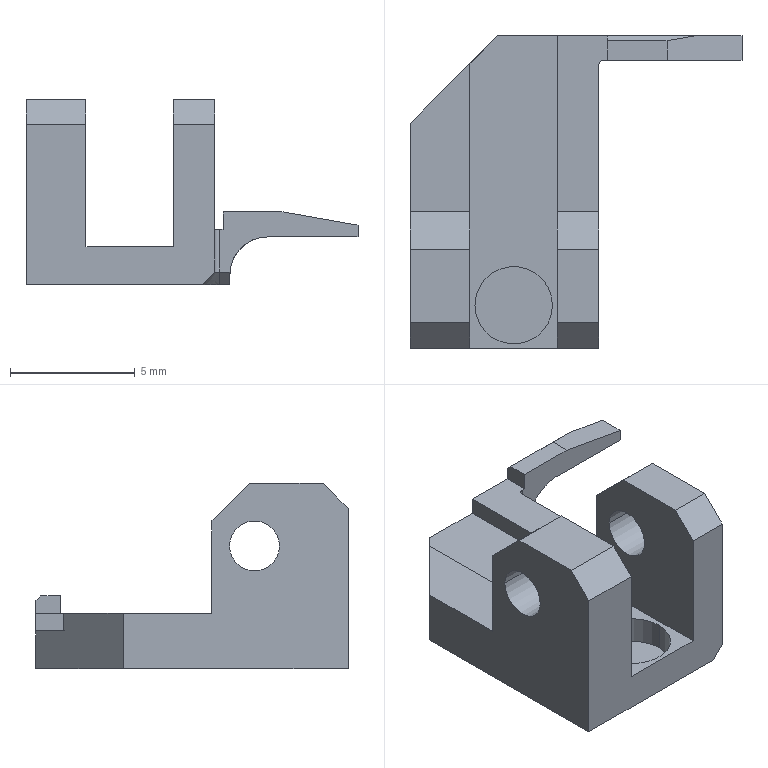Part | NX | 1 solid | 39 faces | box 13.281 x 12.5 x 7.405 mm | volume 256.212 mm3 | plane 30 | cylinder 8 | cone 1 | commonest cylinder face diameters 2 x4 3.1 x2 0.4 x1 3 x1
STEP:
#1=CARTESIAN_POINT('',(-42.479,-42.729,-0.8259));
#2=VERTEX_POINT('',#1);
#3=CARTESIAN_POINT('',(-42.479,-43.716,-0.8259));
#4=VERTEX_POINT('',#3);
#5=CARTESIAN_POINT('',(-42.479,-43.322,-0.8259));
#6=DIRECTION('',(0.,-1.,0.));
#7=VECTOR('',#6,1000.);
#8=LINE('',#5,#7);
#9=EDGE_CURVE('',#2,#4,#8,.T.);
#10=ORIENTED_EDGE('',*,*,#9,.T.);
#11=CARTESIAN_POINT('',(-42.479,-43.716,-1.297));
#12=VERTEX_POINT('',#11);
#13=CARTESIAN_POINT('',(-42.479,-43.716,-2.097));
#14=DIRECTION('',(0.,0.,1.));
#15=VECTOR('',#14,1000.);
#16=LINE('',#13,#15);
#17=EDGE_CURVE('',#12,#4,#16,.T.);
#18=ORIENTED_EDGE('',*,*,#17,.F.);
#19=CARTESIAN_POINT('',(-42.479,-42.729,-1.297));
#20=VERTEX_POINT('',#19);
#21=CARTESIAN_POINT('',(-42.479,-42.161,-1.297));
#22=DIRECTION('',(0.,1.,0.));
#23=VECTOR('',#22,1000.);
#24=LINE('',#21,#23);
#25=EDGE_CURVE('',#12,#20,#24,.T.);
#26=ORIENTED_EDGE('',*,*,#25,.T.);
#27=CARTESIAN_POINT('',(-42.479,-42.729,-2.097));
#28=DIRECTION('',(0.,0.,-1.));
#29=VECTOR('',#28,1000.);
#30=LINE('',#27,#29);
#31=EDGE_CURVE('',#2,#20,#30,.T.);
#32=ORIENTED_EDGE('',*,*,#31,.F.);
#33=EDGE_LOOP('',(#10,#18,#26,#32));
#34=FACE_BOUND('',#33,.T.);
#35=CARTESIAN_POINT('',(-42.479,-43.677,-2.097));
#36=DIRECTION('',(1.,0.,0.));
#37=DIRECTION('',(0.,0.,1.));
#38=AXIS2_PLACEMENT_3D('',#35,#36,#37);
#39=PLANE('',#38);
#40=ADVANCED_FACE('',(#34),#39,.T.);
#41=CARTESIAN_POINT('',(-47.879,-43.716,-0.9969));
#42=VERTEX_POINT('',#41);
#43=CARTESIAN_POINT('',(-47.879,-43.716,-0.2969));
#44=VERTEX_POINT('',#43);
#45=CARTESIAN_POINT('',(-47.879,-43.716,-2.097));
#46=DIRECTION('',(0.,0.,1.));
#47=VECTOR('',#46,1000.);
#48=LINE('',#45,#47);
#49=EDGE_CURVE('',#42,#44,#48,.T.);
#50=ORIENTED_EDGE('',*,*,#49,.T.);
#51=CARTESIAN_POINT('',(-47.879,-42.929,-0.2969));
#52=VERTEX_POINT('',#51);
#53=CARTESIAN_POINT('',(-47.879,-42.161,-0.2969));
#54=DIRECTION('',(0.,-1.,0.));
#55=VECTOR('',#54,1000.);
#56=LINE('',#53,#55);
#57=EDGE_CURVE('',#52,#44,#56,.T.);
#58=ORIENTED_EDGE('',*,*,#57,.F.);
#59=CARTESIAN_POINT('',(-47.879,-42.729,-0.4969));
#60=VERTEX_POINT('',#59);
#61=CARTESIAN_POINT('',(-47.879,-42.161,-1.065));
#62=DIRECTION('',(0.,0.7071,-0.7071));
#63=VECTOR('',#62,1000.);
#64=LINE('',#61,#63);
#65=EDGE_CURVE('',#52,#60,#64,.T.);
#66=ORIENTED_EDGE('',*,*,#65,.T.);
#67=CARTESIAN_POINT('',(-47.879,-42.729,-0.9969));
#68=VERTEX_POINT('',#67);
#69=CARTESIAN_POINT('',(-47.879,-42.729,-2.097));
#70=DIRECTION('',(0.,0.,-1.));
#71=VECTOR('',#70,1000.);
#72=LINE('',#69,#71);
#73=EDGE_CURVE('',#60,#68,#72,.T.);
#74=ORIENTED_EDGE('',*,*,#73,.T.);
#75=CARTESIAN_POINT('',(-47.879,-42.161,-0.9969));
#76=DIRECTION('',(0.,-1.,0.));
#77=VECTOR('',#76,1000.);
#78=LINE('',#75,#77);
#79=EDGE_CURVE('',#68,#42,#78,.T.);
#80=ORIENTED_EDGE('',*,*,#79,.T.);
#81=EDGE_LOOP('',(#50,#58,#66,#74,#80));
#82=FACE_BOUND('',#81,.T.);
#83=CARTESIAN_POINT('',(-47.879,-42.677,-2.097));
#84=DIRECTION('',(-1.,0.,0.));
#85=DIRECTION('',(0.,1.,0.));
#86=AXIS2_PLACEMENT_3D('',#83,#84,#85);
#87=PLANE('',#86);
#88=ADVANCED_FACE('',(#82),#87,.T.);
#89=CARTESIAN_POINT('',(-53.36,-43.829,-1.697));
#90=VERTEX_POINT('',#89);
#91=CARTESIAN_POINT('',(-53.36,-55.229,-1.697));
#92=VERTEX_POINT('',#91);
#93=CARTESIAN_POINT('',(-53.36,-42.161,-1.697));
#94=DIRECTION('',(0.,-1.,0.));
#95=VECTOR('',#94,1000.);
#96=LINE('',#93,#95);
#97=EDGE_CURVE('',#90,#92,#96,.T.);
#98=ORIENTED_EDGE('',*,*,#97,.F.);
#99=CARTESIAN_POINT('',(-53.36,-43.829,-0.9969));
#100=VERTEX_POINT('',#99);
#101=CARTESIAN_POINT('',(-53.36,-43.829,-2.097));
#102=DIRECTION('',(0.,0.,-1.));
#103=VECTOR('',#102,1000.);
#104=LINE('',#101,#103);
#105=EDGE_CURVE('',#100,#90,#104,.T.);
#106=ORIENTED_EDGE('',*,*,#105,.F.);
#107=CARTESIAN_POINT('',(-53.36,-49.779,-0.9969));
#108=VERTEX_POINT('',#107);
#109=CARTESIAN_POINT('',(-53.36,-42.161,-0.9969));
#110=DIRECTION('',(0.,-1.,0.));
#111=VECTOR('',#110,1000.);
#112=LINE('',#109,#111);
#113=EDGE_CURVE('',#100,#108,#112,.T.);
#114=ORIENTED_EDGE('',*,*,#113,.T.);
#115=CARTESIAN_POINT('',(-53.36,-49.779,2.703));
#116=VERTEX_POINT('',#115);
#117=CARTESIAN_POINT('',(-53.36,-49.779,-2.097));
#118=DIRECTION('',(0.,0.,-1.));
#119=VECTOR('',#118,1000.);
#120=LINE('',#117,#119);
#121=EDGE_CURVE('',#116,#108,#120,.T.);
#122=ORIENTED_EDGE('',*,*,#121,.F.);
#123=CARTESIAN_POINT('',(-53.36,-51.279,4.203));
#124=VERTEX_POINT('',#123);
#125=CARTESIAN_POINT('',(-53.36,-44.979,-2.097));
#126=DIRECTION('',(0.,-0.7071,0.7071));
#127=VECTOR('',#126,1000.);
#128=LINE('',#125,#127);
#129=EDGE_CURVE('',#116,#124,#128,.T.);
#130=ORIENTED_EDGE('',*,*,#129,.T.);
#131=CARTESIAN_POINT('',(-53.36,-54.229,4.203));
#132=VERTEX_POINT('',#131);
#133=CARTESIAN_POINT('',(-53.36,-42.161,4.203));
#134=DIRECTION('',(0.,1.,0.));
#135=VECTOR('',#134,1000.);
#136=LINE('',#133,#135);
#137=EDGE_CURVE('',#132,#124,#136,.T.);
#138=ORIENTED_EDGE('',*,*,#137,.F.);
#139=CARTESIAN_POINT('',(-53.36,-55.229,3.203));
#140=VERTEX_POINT('',#139);
#141=CARTESIAN_POINT('',(-53.36,-60.529,-2.097));
#142=DIRECTION('',(0.,-0.7071,-0.7071));
#143=VECTOR('',#142,1000.);
#144=LINE('',#141,#143);
#145=EDGE_CURVE('',#132,#140,#144,.T.);
#146=ORIENTED_EDGE('',*,*,#145,.T.);
#147=CARTESIAN_POINT('',(-53.36,-55.229,-2.097));
#148=DIRECTION('',(0.,0.,1.));
#149=VECTOR('',#148,1000.);
#150=LINE('',#147,#149);
#151=EDGE_CURVE('',#92,#140,#150,.T.);
#152=ORIENTED_EDGE('',*,*,#151,.F.);
#153=EDGE_LOOP('',(#98,#106,#114,#122,#130,#138,#146,#152));
#154=FACE_BOUND('',#153,.T.);
#155=CARTESIAN_POINT('',(-53.36,-50.479,1.703));
#156=VERTEX_POINT('',#155);
#157=CARTESIAN_POINT('',(-53.36,-52.479,1.703));
#158=VERTEX_POINT('',#157);
#159=CARTESIAN_POINT('',(-53.36,-51.479,1.703));
#160=DIRECTION('',(-1.,0.,0.));
#161=DIRECTION('',(0.,-1.,0.));
#162=AXIS2_PLACEMENT_3D('',#159,#160,#161);
#163=CIRCLE('',#162,1.);
#164=EDGE_CURVE('',#156,#158,#163,.T.);
#165=ORIENTED_EDGE('',*,*,#164,.T.);
#166=CARTESIAN_POINT('',(-53.36,-51.479,1.703));
#167=DIRECTION('',(-1.,0.,0.));
#168=DIRECTION('',(0.,-1.,0.));
#169=AXIS2_PLACEMENT_3D('',#166,#167,#168);
#170=CIRCLE('',#169,1.);
#171=EDGE_CURVE('',#158,#156,#170,.T.);
#172=ORIENTED_EDGE('',*,*,#171,.T.);
#173=EDGE_LOOP('',(#165,#172));
#174=FACE_BOUND('',#173,.T.);
#175=CARTESIAN_POINT('',(-53.36,-41.455,-0.9969));
#176=DIRECTION('',(-1.,0.,0.));
#177=DIRECTION('',(0.,0.,1.));
#178=AXIS2_PLACEMENT_3D('',#175,#176,#177);
#179=PLANE('',#178);
#180=ADVANCED_FACE('',(#154,#174),#179,.F.);
#181=CARTESIAN_POINT('',(-49.86,-42.729,-1.697));
#182=VERTEX_POINT('',#181);
#183=CARTESIAN_POINT('',(-52.26,-42.729,-1.697));
#184=VERTEX_POINT('',#183);
#185=CARTESIAN_POINT('',(-49.458,-42.729,-1.697));
#186=DIRECTION('',(-1.,0.,0.));
#187=VECTOR('',#186,1000.);
#188=LINE('',#185,#187);
#189=EDGE_CURVE('',#182,#184,#188,.T.);
#190=ORIENTED_EDGE('',*,*,#189,.F.);
#191=CARTESIAN_POINT('',(-49.86,-42.729,-0.9969));
#192=VERTEX_POINT('',#191);
#193=CARTESIAN_POINT('',(-49.86,-42.729,-2.097));
#194=DIRECTION('',(0.,0.,-1.));
#195=VECTOR('',#194,1000.);
#196=LINE('',#193,#195);
#197=EDGE_CURVE('',#192,#182,#196,.T.);
#198=ORIENTED_EDGE('',*,*,#197,.F.);
#199=CARTESIAN_POINT('',(-49.458,-42.729,-0.9969));
#200=DIRECTION('',(-1.,0.,0.));
#201=VECTOR('',#200,1000.);
#202=LINE('',#199,#201);
#203=EDGE_CURVE('',#68,#192,#202,.T.);
#204=ORIENTED_EDGE('',*,*,#203,.F.);
#205=ORIENTED_EDGE('',*,*,#73,.F.);
#206=CARTESIAN_POINT('',(-44.345,-42.729,-0.4969));
#207=VERTEX_POINT('',#206);
#208=CARTESIAN_POINT('',(-49.458,-42.729,-0.4969));
#209=DIRECTION('',(1.,0.,0.));
#210=VECTOR('',#209,1000.);
#211=LINE('',#208,#210);
#212=EDGE_CURVE('',#60,#207,#211,.T.);
#213=ORIENTED_EDGE('',*,*,#212,.T.);
#214=CARTESIAN_POINT('',(-49.458,-42.729,0.4047));
#215=DIRECTION('',(0.9848,0.,-0.1736));
#216=VECTOR('',#215,1000.);
#217=LINE('',#214,#216);
#218=EDGE_CURVE('',#207,#2,#217,.T.);
#219=ORIENTED_EDGE('',*,*,#218,.T.);
#220=ORIENTED_EDGE('',*,*,#31,.T.);
#221=CARTESIAN_POINT('',(-46.102,-42.729,-1.297));
#222=VERTEX_POINT('',#221);
#223=CARTESIAN_POINT('',(-49.458,-42.729,-1.297));
#224=DIRECTION('',(-1.,0.,0.));
#225=VECTOR('',#224,1000.);
#226=LINE('',#223,#225);
#227=EDGE_CURVE('',#20,#222,#226,.T.);
#228=ORIENTED_EDGE('',*,*,#227,.T.);
#229=CARTESIAN_POINT('',(-47.602,-42.729,-2.797));
#230=VERTEX_POINT('',#229);
#231=CARTESIAN_POINT('',(-46.102,-42.729,-2.797));
#232=DIRECTION('',(0.,1.,0.));
#233=DIRECTION('',(-1.,0.,0.));
#234=AXIS2_PLACEMENT_3D('',#231,#232,#233);
#235=CIRCLE('',#234,1.5);
#236=EDGE_CURVE('',#230,#222,#235,.T.);
#237=ORIENTED_EDGE('',*,*,#236,.F.);
#238=CARTESIAN_POINT('',(-47.602,-42.729,-3.201));
#239=VERTEX_POINT('',#238);
#240=CARTESIAN_POINT('',(-47.602,-42.729,-2.097));
#241=DIRECTION('',(0.,0.,1.));
#242=VECTOR('',#241,1000.);
#243=LINE('',#240,#242);
#244=EDGE_CURVE('',#239,#230,#243,.T.);
#245=ORIENTED_EDGE('',*,*,#244,.F.);
#246=CARTESIAN_POINT('',(-52.26,-42.729,-3.201));
#247=VERTEX_POINT('',#246);
#248=CARTESIAN_POINT('',(-49.458,-42.729,-3.201));
#249=DIRECTION('',(-1.,0.,0.));
#250=VECTOR('',#249,1000.);
#251=LINE('',#248,#250);
#252=EDGE_CURVE('',#239,#247,#251,.T.);
#253=ORIENTED_EDGE('',*,*,#252,.T.);
#254=CARTESIAN_POINT('',(-52.26,-42.729,-2.097));
#255=DIRECTION('',(0.,0.,1.));
#256=VECTOR('',#255,1000.);
#257=LINE('',#254,#256);
#258=EDGE_CURVE('',#247,#184,#257,.T.);
#259=ORIENTED_EDGE('',*,*,#258,.T.);
#260=EDGE_LOOP('',(#190,#198,#204,#205,#213,#219,#220,#228,#237,#245,#253,#259));
#261=FACE_BOUND('',#260,.T.);
#262=CARTESIAN_POINT('',(-40.479,-42.729,-2.097));
#263=DIRECTION('',(0.,1.,0.));
#264=DIRECTION('',(0.,0.,-1.));
#265=AXIS2_PLACEMENT_3D('',#262,#263,#264);
#266=PLANE('',#265);
#267=ADVANCED_FACE('',(#261),#266,.T.);
#268=CARTESIAN_POINT('',(-48.01,-43.716,-2.701));
#269=VERTEX_POINT('',#268);
#270=CARTESIAN_POINT('',(-47.599,-43.716,-2.701));
#271=VERTEX_POINT('',#270);
#272=CARTESIAN_POINT('',(-47.806,-43.716,-2.701));
#273=DIRECTION('',(1.,0.,0.));
#274=VECTOR('',#273,1000.);
#275=LINE('',#272,#274);
#276=EDGE_CURVE('',#269,#271,#275,.T.);
#277=ORIENTED_EDGE('',*,*,#276,.T.);
#278=CARTESIAN_POINT('',(-46.102,-43.716,-1.297));
#279=VERTEX_POINT('',#278);
#280=CARTESIAN_POINT('',(-46.102,-43.716,-2.797));
#281=DIRECTION('',(0.,1.,0.));
#282=DIRECTION('',(-1.,0.,0.));
#283=AXIS2_PLACEMENT_3D('',#280,#281,#282);
#284=CIRCLE('',#283,1.5);
#285=EDGE_CURVE('',#271,#279,#284,.T.);
#286=ORIENTED_EDGE('',*,*,#285,.T.);
#287=CARTESIAN_POINT('',(-49.458,-43.716,-1.297));
#288=DIRECTION('',(1.,0.,0.));
#289=VECTOR('',#288,1000.);
#290=LINE('',#287,#289);
#291=EDGE_CURVE('',#279,#12,#290,.T.);
#292=ORIENTED_EDGE('',*,*,#291,.T.);
#293=ORIENTED_EDGE('',*,*,#17,.T.);
#294=CARTESIAN_POINT('',(-45.479,-43.716,-0.2969));
#295=VERTEX_POINT('',#294);
#296=CARTESIAN_POINT('',(-49.458,-43.716,0.4047));
#297=DIRECTION('',(-0.9848,0.,0.1736));
#298=VECTOR('',#297,1000.);
#299=LINE('',#296,#298);
#300=EDGE_CURVE('',#4,#295,#299,.T.);
#301=ORIENTED_EDGE('',*,*,#300,.T.);
#302=CARTESIAN_POINT('',(-49.458,-43.716,-0.2969));
#303=DIRECTION('',(-1.,0.,0.));
#304=VECTOR('',#303,1000.);
#305=LINE('',#302,#304);
#306=EDGE_CURVE('',#295,#44,#305,.T.);
#307=ORIENTED_EDGE('',*,*,#306,.T.);
#308=ORIENTED_EDGE('',*,*,#49,.F.);
#309=CARTESIAN_POINT('',(-48.01,-43.716,-0.9969));
#310=VERTEX_POINT('',#309);
#311=CARTESIAN_POINT('',(-49.458,-43.716,-0.9969));
#312=DIRECTION('',(1.,0.,0.));
#313=VECTOR('',#312,1000.);
#314=LINE('',#311,#313);
#315=EDGE_CURVE('',#310,#42,#314,.T.);
#316=ORIENTED_EDGE('',*,*,#315,.F.);
#317=CARTESIAN_POINT('',(-48.01,-43.716,-2.097));
#318=DIRECTION('',(0.,0.,-1.));
#319=VECTOR('',#318,1000.);
#320=LINE('',#317,#319);
#321=EDGE_CURVE('',#310,#269,#320,.T.);
#322=ORIENTED_EDGE('',*,*,#321,.T.);
#323=EDGE_LOOP('',(#277,#286,#292,#293,#301,#307,#308,#316,#322));
#324=FACE_BOUND('',#323,.T.);
#325=CARTESIAN_POINT('',(-49.857,-43.716,-2.975));
#326=DIRECTION('',(0.,-1.,0.));
#327=DIRECTION('',(-1.,0.,0.));
#328=AXIS2_PLACEMENT_3D('',#325,#326,#327);
#329=PLANE('',#328);
#330=ADVANCED_FACE('',(#324),#329,.T.);
#331=CARTESIAN_POINT('',(-48.21,-55.229,-2.701));
#332=VERTEX_POINT('',#331);
#333=CARTESIAN_POINT('',(-48.21,-55.229,3.203));
#334=VERTEX_POINT('',#333);
#335=CARTESIAN_POINT('',(-48.21,-55.229,-2.097));
#336=DIRECTION('',(0.,0.,1.));
#337=VECTOR('',#336,1000.);
#338=LINE('',#335,#337);
#339=EDGE_CURVE('',#332,#334,#338,.T.);
#340=ORIENTED_EDGE('',*,*,#339,.T.);
#341=CARTESIAN_POINT('',(-49.86,-55.229,3.203));
#342=VERTEX_POINT('',#341);
#343=CARTESIAN_POINT('',(-49.035,-55.229,3.203));
#344=DIRECTION('',(1.,0.,0.));
#345=VECTOR('',#344,1000.);
#346=LINE('',#343,#345);
#347=EDGE_CURVE('',#342,#334,#346,.T.);
#348=ORIENTED_EDGE('',*,*,#347,.F.);
#349=CARTESIAN_POINT('',(-49.86,-55.229,-1.697));
#350=VERTEX_POINT('',#349);
#351=CARTESIAN_POINT('',(-49.86,-55.229,-2.097));
#352=DIRECTION('',(0.,0.,-1.));
#353=VECTOR('',#352,1000.);
#354=LINE('',#351,#353);
#355=EDGE_CURVE('',#342,#350,#354,.T.);
#356=ORIENTED_EDGE('',*,*,#355,.T.);
#357=CARTESIAN_POINT('',(-49.458,-55.229,-1.697));
#358=DIRECTION('',(-1.,0.,0.));
#359=VECTOR('',#358,1000.);
#360=LINE('',#357,#359);
#361=EDGE_CURVE('',#350,#92,#360,.T.);
#362=ORIENTED_EDGE('',*,*,#361,.T.);
#363=ORIENTED_EDGE('',*,*,#151,.T.);
#364=CARTESIAN_POINT('',(-55.76,-55.229,3.203));
#365=VERTEX_POINT('',#364);
#366=CARTESIAN_POINT('',(-49.458,-55.229,3.203));
#367=DIRECTION('',(1.,0.,0.));
#368=VECTOR('',#367,1000.);
#369=LINE('',#366,#368);
#370=EDGE_CURVE('',#365,#140,#369,.T.);
#371=ORIENTED_EDGE('',*,*,#370,.F.);
#372=CARTESIAN_POINT('',(-55.76,-55.229,-3.201));
#373=VERTEX_POINT('',#372);
#374=CARTESIAN_POINT('',(-55.76,-55.229,-2.097));
#375=DIRECTION('',(0.,0.,-1.));
#376=VECTOR('',#375,1000.);
#377=LINE('',#374,#376);
#378=EDGE_CURVE('',#365,#373,#377,.T.);
#379=ORIENTED_EDGE('',*,*,#378,.T.);
#380=CARTESIAN_POINT('',(-48.71,-55.229,-3.201));
#381=VERTEX_POINT('',#380);
#382=CARTESIAN_POINT('',(-49.458,-55.229,-3.201));
#383=DIRECTION('',(1.,0.,0.));
#384=VECTOR('',#383,1000.);
#385=LINE('',#382,#384);
#386=EDGE_CURVE('',#373,#381,#385,.T.);
#387=ORIENTED_EDGE('',*,*,#386,.T.);
#388=CARTESIAN_POINT('',(-49.458,-55.229,-3.949));
#389=DIRECTION('',(0.7071,0.,0.7071));
#390=VECTOR('',#389,1000.);
#391=LINE('',#388,#390);
#392=EDGE_CURVE('',#381,#332,#391,.T.);
#393=ORIENTED_EDGE('',*,*,#392,.T.);
#394=EDGE_LOOP('',(#340,#348,#356,#362,#363,#371,#379,#387,#393));
#395=FACE_BOUND('',#394,.T.);
#396=CARTESIAN_POINT('',(-46.479,-55.229,-2.097));
#397=DIRECTION('',(0.,-1.,0.));
#398=DIRECTION('',(-1.,0.,0.));
#399=AXIS2_PLACEMENT_3D('',#396,#397,#398);
#400=PLANE('',#399);
#401=ADVANCED_FACE('',(#395),#400,.T.);
#402=CARTESIAN_POINT('',(-47.602,-43.62,-2.797));
#403=VERTEX_POINT('',#402);
#404=CARTESIAN_POINT('',(-47.602,-42.161,-2.797));
#405=DIRECTION('',(0.,1.,0.));
#406=VECTOR('',#405,1000.);
#407=LINE('',#404,#406);
#408=EDGE_CURVE('',#403,#230,#407,.T.);
#409=ORIENTED_EDGE('',*,*,#408,.F.);
#410=CARTESIAN_POINT('',(-47.602,-43.216,-3.201));
#411=VERTEX_POINT('',#410);
#412=CARTESIAN_POINT('',(-47.602,-44.32,-2.097));
#413=DIRECTION('',(0.,0.7071,-0.7071));
#414=VECTOR('',#413,1000.);
#415=LINE('',#412,#414);
#416=EDGE_CURVE('',#403,#411,#415,.T.);
#417=ORIENTED_EDGE('',*,*,#416,.T.);
#418=CARTESIAN_POINT('',(-47.602,-42.161,-3.201));
#419=DIRECTION('',(0.,-1.,0.));
#420=VECTOR('',#419,1000.);
#421=LINE('',#418,#420);
#422=EDGE_CURVE('',#239,#411,#421,.T.);
#423=ORIENTED_EDGE('',*,*,#422,.F.);
#424=ORIENTED_EDGE('',*,*,#244,.T.);
#425=EDGE_LOOP('',(#409,#417,#423,#424));
#426=FACE_BOUND('',#425,.T.);
#427=CARTESIAN_POINT('',(-47.602,-42.161,-2.747));
#428=DIRECTION('',(-1.,0.,0.));
#429=DIRECTION('',(0.,0.,1.));
#430=AXIS2_PLACEMENT_3D('',#427,#428,#429);
#431=PLANE('',#430);
#432=ADVANCED_FACE('',(#426),#431,.F.);
#433=ORIENTED_EDGE('',*,*,#164,.F.);
#434=CARTESIAN_POINT('',(-55.76,-50.479,1.703));
#435=VERTEX_POINT('',#434);
#436=CARTESIAN_POINT('',(-40.131,-50.479,1.703));
#437=DIRECTION('',(-1.,0.,0.));
#438=VECTOR('',#437,1000.);
#439=LINE('',#436,#438);
#440=EDGE_CURVE('',#435,#156,#439,.F.);
#441=ORIENTED_EDGE('',*,*,#440,.F.);
#442=CARTESIAN_POINT('',(-55.76,-52.479,1.703));
#443=VERTEX_POINT('',#442);
#444=CARTESIAN_POINT('',(-55.76,-51.479,1.703));
#445=DIRECTION('',(-1.,0.,0.));
#446=DIRECTION('',(0.,-1.,0.));
#447=AXIS2_PLACEMENT_3D('',#444,#445,#446);
#448=CIRCLE('',#447,1.);
#449=EDGE_CURVE('',#435,#443,#448,.T.);
#450=ORIENTED_EDGE('',*,*,#449,.T.);
#451=CARTESIAN_POINT('',(-40.131,-52.479,1.703));
#452=DIRECTION('',(-1.,0.,0.));
#453=VECTOR('',#452,1000.);
#454=LINE('',#451,#453);
#455=EDGE_CURVE('',#443,#158,#454,.F.);
#456=ORIENTED_EDGE('',*,*,#455,.T.);
#457=EDGE_LOOP('',(#433,#441,#450,#456));
#458=FACE_BOUND('',#457,.T.);
#459=CARTESIAN_POINT('',(-40.131,-51.479,1.703));
#460=DIRECTION('',(-1.,0.,0.));
#461=DIRECTION('',(0.,-1.,0.));
#462=AXIS2_PLACEMENT_3D('',#459,#460,#461);
#463=CYLINDRICAL_SURFACE('',#462,1.);
#464=ADVANCED_FACE('',(#458),#463,.F.);
#465=CARTESIAN_POINT('',(-48.21,-43.916,-2.701));
#466=VERTEX_POINT('',#465);
#467=CARTESIAN_POINT('',(-48.01,-43.916,-2.701));
#468=DIRECTION('',(0.,0.,-1.));
#469=DIRECTION('',(-1.,0.,0.));
#470=AXIS2_PLACEMENT_3D('',#467,#468,#469);
#471=CIRCLE('',#470,0.2);
#472=EDGE_CURVE('',#466,#269,#471,.T.);
#473=ORIENTED_EDGE('',*,*,#472,.T.);
#474=ORIENTED_EDGE('',*,*,#321,.F.);
#475=CARTESIAN_POINT('',(-48.21,-43.916,-0.9969));
#476=VERTEX_POINT('',#475);
#477=CARTESIAN_POINT('',(-48.01,-43.916,-0.9969));
#478=DIRECTION('',(0.,0.,-1.));
#479=DIRECTION('',(-1.,0.,0.));
#480=AXIS2_PLACEMENT_3D('',#477,#478,#479);
#481=CIRCLE('',#480,0.2);
#482=EDGE_CURVE('',#476,#310,#481,.T.);
#483=ORIENTED_EDGE('',*,*,#482,.F.);
#484=CARTESIAN_POINT('',(-48.21,-43.916,-2.097));
#485=DIRECTION('',(0.,0.,-1.));
#486=VECTOR('',#485,1000.);
#487=LINE('',#484,#486);
#488=EDGE_CURVE('',#476,#466,#487,.T.);
#489=ORIENTED_EDGE('',*,*,#488,.T.);
#490=EDGE_LOOP('',(#473,#474,#483,#489));
#491=FACE_BOUND('',#490,.T.);
#492=CARTESIAN_POINT('',(-48.01,-43.916,-2.097));
#493=DIRECTION('',(0.,0.,-1.));
#494=DIRECTION('',(-1.,0.,0.));
#495=AXIS2_PLACEMENT_3D('',#492,#493,#494);
#496=CYLINDRICAL_SURFACE('',#495,0.2);
#497=ADVANCED_FACE('',(#491),#496,.F.);
#498=ORIENTED_EDGE('',*,*,#276,.F.);
#499=CARTESIAN_POINT('',(-48.01,-43.216,-3.201));
#500=VERTEX_POINT('',#499);
#501=CARTESIAN_POINT('',(-48.01,-43.716,-2.701));
#502=DIRECTION('',(0.,0.7071,-0.7071));
#503=VECTOR('',#502,1000.);
#504=LINE('',#501,#503);
#505=EDGE_CURVE('',#269,#500,#504,.T.);
#506=ORIENTED_EDGE('',*,*,#505,.T.);
#507=CARTESIAN_POINT('',(-47.806,-43.216,-3.201));
#508=DIRECTION('',(1.,0.,0.));
#509=VECTOR('',#508,1000.);
#510=LINE('',#507,#509);
#511=EDGE_CURVE('',#500,#411,#510,.T.);
#512=ORIENTED_EDGE('',*,*,#511,.T.);
#513=ORIENTED_EDGE('',*,*,#416,.F.);
#514=CARTESIAN_POINT('',(-47.599,-43.716,-2.701));
#515=CARTESIAN_POINT('',(-47.601,-43.684,-2.733));
#516=CARTESIAN_POINT('',(-47.602,-43.652,-2.765));
#517=CARTESIAN_POINT('',(-47.602,-43.62,-2.797));
#518=(BOUNDED_CURVE()B_SPLINE_CURVE(3,(#514,#515,#516,#517),.UNSPECIFIED.,.F.,.F.)B_SPLINE_CURVE_WITH_KNOTS((4,4),(4.649,4.712),.UNSPECIFIED.)CURVE()GEOMETRIC_REPRESENTATION_ITEM()RATIONAL_B_SPLINE_CURVE((1.,0.9997,0.9997,1.))REPRESENTATION_ITEM(''));
#519=EDGE_CURVE('',#271,#403,#518,.T.);
#520=ORIENTED_EDGE('',*,*,#519,.F.);
#521=EDGE_LOOP('',(#498,#506,#512,#513,#520));
#522=FACE_BOUND('',#521,.T.);
#523=CARTESIAN_POINT('',(-47.806,-43.466,-2.951));
#524=DIRECTION('',(0.,-0.7071,-0.7071));
#525=DIRECTION('',(0.,-0.7071,0.7071));
#526=AXIS2_PLACEMENT_3D('',#523,#524,#525);
#527=PLANE('',#526);
#528=ADVANCED_FACE('',(#522),#527,.T.);
#529=ORIENTED_EDGE('',*,*,#472,.F.);
#530=CARTESIAN_POINT('',(-48.71,-43.916,-3.201));
#531=VERTEX_POINT('',#530);
#532=CARTESIAN_POINT('',(-48.21,-43.916,-2.701));
#533=DIRECTION('',(-0.7071,0.,-0.7071));
#534=VECTOR('',#533,1000.);
#535=LINE('',#532,#534);
#536=EDGE_CURVE('',#466,#531,#535,.T.);
#537=ORIENTED_EDGE('',*,*,#536,.T.);
#538=CARTESIAN_POINT('',(-48.01,-43.916,-3.201));
#539=DIRECTION('',(0.,0.,-1.));
#540=DIRECTION('',(-1.,0.,0.));
#541=AXIS2_PLACEMENT_3D('',#538,#539,#540);
#542=CIRCLE('',#541,0.7);
#543=EDGE_CURVE('',#531,#500,#542,.T.);
#544=ORIENTED_EDGE('',*,*,#543,.T.);
#545=ORIENTED_EDGE('',*,*,#505,.F.);
#546=EDGE_LOOP('',(#529,#537,#544,#545));
#547=FACE_BOUND('',#546,.T.);
#548=CARTESIAN_POINT('',(-48.01,-43.916,-2.701));
#549=DIRECTION('',(0.,0.,-1.));
#550=DIRECTION('',(-1.,0.,0.));
#551=AXIS2_PLACEMENT_3D('',#548,#549,#550);
#552=CONICAL_SURFACE('',#551,0.2,0.7854);
#553=ADVANCED_FACE('',(#547),#552,.F.);
#554=ORIENTED_EDGE('',*,*,#408,.T.);
#555=ORIENTED_EDGE('',*,*,#236,.T.);
#556=CARTESIAN_POINT('',(-46.102,-42.161,-1.297));
#557=DIRECTION('',(0.,1.,0.));
#558=VECTOR('',#557,1000.);
#559=LINE('',#556,#558);
#560=EDGE_CURVE('',#279,#222,#559,.T.);
#561=ORIENTED_EDGE('',*,*,#560,.F.);
#562=ORIENTED_EDGE('',*,*,#285,.F.);
#563=ORIENTED_EDGE('',*,*,#519,.T.);
#564=EDGE_LOOP('',(#554,#555,#561,#562,#563));
#565=FACE_BOUND('',#564,.T.);
#566=CARTESIAN_POINT('',(-46.102,-42.161,-2.797));
#567=DIRECTION('',(0.,1.,0.));
#568=DIRECTION('',(-1.,0.,0.));
#569=AXIS2_PLACEMENT_3D('',#566,#567,#568);
#570=CYLINDRICAL_SURFACE('',#569,1.5);
#571=ADVANCED_FACE('',(#565),#570,.F.);
#572=ORIENTED_EDGE('',*,*,#455,.F.);
#573=CARTESIAN_POINT('',(-55.76,-51.479,1.703));
#574=DIRECTION('',(-1.,0.,0.));
#575=DIRECTION('',(0.,-1.,0.));
#576=AXIS2_PLACEMENT_3D('',#573,#574,#575);
#577=CIRCLE('',#576,1.);
#578=EDGE_CURVE('',#443,#435,#577,.T.);
#579=ORIENTED_EDGE('',*,*,#578,.T.);
#580=ORIENTED_EDGE('',*,*,#440,.T.);
#581=ORIENTED_EDGE('',*,*,#171,.F.);
#582=EDGE_LOOP('',(#572,#579,#580,#581));
#583=FACE_BOUND('',#582,.T.);
#584=CARTESIAN_POINT('',(-40.131,-51.479,1.703));
#585=DIRECTION('',(-1.,0.,0.));
#586=DIRECTION('',(0.,-1.,0.));
#587=AXIS2_PLACEMENT_3D('',#584,#585,#586);
#588=CYLINDRICAL_SURFACE('',#587,1.);
#589=ADVANCED_FACE('',(#583),#588,.F.);
#590=ORIENTED_EDGE('',*,*,#511,.F.);
#591=ORIENTED_EDGE('',*,*,#543,.F.);
#592=CARTESIAN_POINT('',(-48.71,-49.572,-3.201));
#593=DIRECTION('',(0.,-1.,0.));
#594=VECTOR('',#593,1000.);
#595=LINE('',#592,#594);
#596=EDGE_CURVE('',#531,#381,#595,.T.);
#597=ORIENTED_EDGE('',*,*,#596,.T.);
#598=ORIENTED_EDGE('',*,*,#386,.F.);
#599=CARTESIAN_POINT('',(-55.76,-46.229,-3.201));
#600=VERTEX_POINT('',#599);
#601=CARTESIAN_POINT('',(-55.76,-42.161,-3.201));
#602=DIRECTION('',(0.,-1.,0.));
#603=VECTOR('',#602,1000.);
#604=LINE('',#601,#603);
#605=EDGE_CURVE('',#600,#373,#604,.T.);
#606=ORIENTED_EDGE('',*,*,#605,.F.);
#607=CARTESIAN_POINT('',(-51.693,-42.161,-3.201));
#608=DIRECTION('',(0.7071,0.7071,0.));
#609=VECTOR('',#608,1000.);
#610=LINE('',#607,#609);
#611=EDGE_CURVE('',#600,#247,#610,.T.);
#612=ORIENTED_EDGE('',*,*,#611,.T.);
#613=ORIENTED_EDGE('',*,*,#252,.F.);
#614=ORIENTED_EDGE('',*,*,#422,.T.);
#615=EDGE_LOOP('',(#590,#591,#597,#598,#606,#612,#613,#614));
#616=FACE_BOUND('',#615,.T.);
#617=CARTESIAN_POINT('',(-49.458,-42.161,-3.201));
#618=DIRECTION('',(0.,0.,-1.));
#619=DIRECTION('',(0.,-1.,0.));
#620=AXIS2_PLACEMENT_3D('',#617,#618,#619);
#621=PLANE('',#620);
#622=ADVANCED_FACE('',(#616),#621,.T.);
#623=CARTESIAN_POINT('',(-55.76,-46.229,-0.9969));
#624=VERTEX_POINT('',#623);
#625=CARTESIAN_POINT('',(-55.76,-46.229,-2.097));
#626=DIRECTION('',(0.,0.,1.));
#627=VECTOR('',#626,1000.);
#628=LINE('',#625,#627);
#629=EDGE_CURVE('',#600,#624,#628,.T.);
#630=ORIENTED_EDGE('',*,*,#629,.F.);
#631=ORIENTED_EDGE('',*,*,#605,.T.);
#632=ORIENTED_EDGE('',*,*,#378,.F.);
#633=CARTESIAN_POINT('',(-55.76,-54.229,4.203));
#634=VERTEX_POINT('',#633);
#635=CARTESIAN_POINT('',(-55.76,-60.529,-2.097));
#636=DIRECTION('',(0.,-0.7071,-0.7071));
#637=VECTOR('',#636,1000.);
#638=LINE('',#635,#637);
#639=EDGE_CURVE('',#634,#365,#638,.T.);
#640=ORIENTED_EDGE('',*,*,#639,.F.);
#641=CARTESIAN_POINT('',(-55.76,-51.279,4.203));
#642=VERTEX_POINT('',#641);
#643=CARTESIAN_POINT('',(-55.76,-42.161,4.203));
#644=DIRECTION('',(0.,-1.,0.));
#645=VECTOR('',#644,1000.);
#646=LINE('',#643,#645);
#647=EDGE_CURVE('',#642,#634,#646,.T.);
#648=ORIENTED_EDGE('',*,*,#647,.F.);
#649=CARTESIAN_POINT('',(-55.76,-49.779,2.703));
#650=VERTEX_POINT('',#649);
#651=CARTESIAN_POINT('',(-55.76,-44.979,-2.097));
#652=DIRECTION('',(0.,-0.7071,0.7071));
#653=VECTOR('',#652,1000.);
#654=LINE('',#651,#653);
#655=EDGE_CURVE('',#650,#642,#654,.T.);
#656=ORIENTED_EDGE('',*,*,#655,.F.);
#657=CARTESIAN_POINT('',(-55.76,-49.779,-0.9969));
#658=VERTEX_POINT('',#657);
#659=CARTESIAN_POINT('',(-55.76,-49.779,-2.097));
#660=DIRECTION('',(0.,0.,1.));
#661=VECTOR('',#660,1000.);
#662=LINE('',#659,#661);
#663=EDGE_CURVE('',#658,#650,#662,.T.);
#664=ORIENTED_EDGE('',*,*,#663,.F.);
#665=CARTESIAN_POINT('',(-55.76,-42.161,-0.9969));
#666=DIRECTION('',(0.,-1.,0.));
#667=VECTOR('',#666,1000.);
#668=LINE('',#665,#667);
#669=EDGE_CURVE('',#624,#658,#668,.T.);
#670=ORIENTED_EDGE('',*,*,#669,.F.);
#671=EDGE_LOOP('',(#630,#631,#632,#640,#648,#656,#664,#670));
#672=FACE_BOUND('',#671,.T.);
#673=ORIENTED_EDGE('',*,*,#449,.F.);
#674=ORIENTED_EDGE('',*,*,#578,.F.);
#675=EDGE_LOOP('',(#673,#674));
#676=FACE_BOUND('',#675,.T.);
#677=CARTESIAN_POINT('',(-55.76,-43.105,-3.373));
#678=DIRECTION('',(-1.,0.,0.));
#679=DIRECTION('',(0.,1.,0.));
#680=AXIS2_PLACEMENT_3D('',#677,#678,#679);
#681=PLANE('',#680);
#682=ADVANCED_FACE('',(#672,#676),#681,.T.);
#683=ORIENTED_EDGE('',*,*,#79,.F.);
#684=ORIENTED_EDGE('',*,*,#203,.T.);
#685=CARTESIAN_POINT('',(-49.86,-49.779,-0.9969));
#686=VERTEX_POINT('',#685);
#687=CARTESIAN_POINT('',(-49.86,-42.161,-0.9969));
#688=DIRECTION('',(0.,1.,0.));
#689=VECTOR('',#688,1000.);
#690=LINE('',#687,#689);
#691=EDGE_CURVE('',#686,#192,#690,.T.);
#692=ORIENTED_EDGE('',*,*,#691,.F.);
#693=CARTESIAN_POINT('',(-48.21,-49.779,-0.9969));
#694=VERTEX_POINT('',#693);
#695=CARTESIAN_POINT('',(-49.458,-49.779,-0.9969));
#696=DIRECTION('',(-1.,0.,0.));
#697=VECTOR('',#696,1000.);
#698=LINE('',#695,#697);
#699=EDGE_CURVE('',#694,#686,#698,.T.);
#700=ORIENTED_EDGE('',*,*,#699,.F.);
#701=CARTESIAN_POINT('',(-48.21,-42.161,-0.9969));
#702=DIRECTION('',(0.,-1.,0.));
#703=VECTOR('',#702,1000.);
#704=LINE('',#701,#703);
#705=EDGE_CURVE('',#476,#694,#704,.T.);
#706=ORIENTED_EDGE('',*,*,#705,.F.);
#707=ORIENTED_EDGE('',*,*,#482,.T.);
#708=ORIENTED_EDGE('',*,*,#315,.T.);
#709=EDGE_LOOP('',(#683,#684,#692,#700,#706,#707,#708));
#710=FACE_BOUND('',#709,.T.);
#711=CARTESIAN_POINT('',(-46.479,-42.677,-0.9969));
#712=DIRECTION('',(0.,0.,1.));
#713=DIRECTION('',(1.,0.,0.));
#714=AXIS2_PLACEMENT_3D('',#711,#712,#713);
#715=PLANE('',#714);
#716=ADVANCED_FACE('',(#710),#715,.T.);
#717=CARTESIAN_POINT('',(-48.21,-49.572,-2.701));
#718=DIRECTION('',(0.,-1.,0.));
#719=VECTOR('',#718,1000.);
#720=LINE('',#717,#719);
#721=EDGE_CURVE('',#466,#332,#720,.T.);
#722=ORIENTED_EDGE('',*,*,#721,.F.);
#723=ORIENTED_EDGE('',*,*,#488,.F.);
#724=ORIENTED_EDGE('',*,*,#705,.T.);
#725=CARTESIAN_POINT('',(-48.21,-49.779,2.703));
#726=VERTEX_POINT('',#725);
#727=CARTESIAN_POINT('',(-48.21,-49.779,-2.097));
#728=DIRECTION('',(0.,0.,-1.));
#729=VECTOR('',#728,1000.);
#730=LINE('',#727,#729);
#731=EDGE_CURVE('',#726,#694,#730,.T.);
#732=ORIENTED_EDGE('',*,*,#731,.F.);
#733=CARTESIAN_POINT('',(-48.21,-51.279,4.203));
#734=VERTEX_POINT('',#733);
#735=CARTESIAN_POINT('',(-48.21,-44.979,-2.097));
#736=DIRECTION('',(0.,-0.7071,0.7071));
#737=VECTOR('',#736,1000.);
#738=LINE('',#735,#737);
#739=EDGE_CURVE('',#726,#734,#738,.T.);
#740=ORIENTED_EDGE('',*,*,#739,.T.);
#741=CARTESIAN_POINT('',(-48.21,-54.229,4.203));
#742=VERTEX_POINT('',#741);
#743=CARTESIAN_POINT('',(-48.21,-42.161,4.203));
#744=DIRECTION('',(0.,-1.,0.));
#745=VECTOR('',#744,1000.);
#746=LINE('',#743,#745);
#747=EDGE_CURVE('',#734,#742,#746,.T.);
#748=ORIENTED_EDGE('',*,*,#747,.T.);
#749=CARTESIAN_POINT('',(-48.21,-60.529,-2.097));
#750=DIRECTION('',(0.,-0.7071,-0.7071));
#751=VECTOR('',#750,1000.);
#752=LINE('',#749,#751);
#753=EDGE_CURVE('',#742,#334,#752,.T.);
#754=ORIENTED_EDGE('',*,*,#753,.T.);
#755=ORIENTED_EDGE('',*,*,#339,.F.);
#756=EDGE_LOOP('',(#722,#723,#724,#732,#740,#748,#754,#755));
#757=FACE_BOUND('',#756,.T.);
#758=CARTESIAN_POINT('',(-48.21,-50.479,1.703));
#759=VERTEX_POINT('',#758);
#760=CARTESIAN_POINT('',(-48.21,-52.479,1.703));
#761=VERTEX_POINT('',#760);
#762=CARTESIAN_POINT('',(-48.21,-51.479,1.703));
#763=DIRECTION('',(-1.,0.,0.));
#764=DIRECTION('',(0.,-1.,0.));
#765=AXIS2_PLACEMENT_3D('',#762,#763,#764);
#766=CIRCLE('',#765,1.);
#767=EDGE_CURVE('',#759,#761,#766,.T.);
#768=ORIENTED_EDGE('',*,*,#767,.T.);
#769=CARTESIAN_POINT('',(-48.21,-51.479,1.703));
#770=DIRECTION('',(-1.,0.,0.));
#771=DIRECTION('',(0.,-1.,0.));
#772=AXIS2_PLACEMENT_3D('',#769,#770,#771);
#773=CIRCLE('',#772,1.);
#774=EDGE_CURVE('',#761,#759,#773,.T.);
#775=ORIENTED_EDGE('',*,*,#774,.T.);
#776=EDGE_LOOP('',(#768,#775));
#777=FACE_BOUND('',#776,.T.);
#778=CARTESIAN_POINT('',(-48.21,-45.316,3.503));
#779=DIRECTION('',(-1.,0.,0.));
#780=DIRECTION('',(0.,0.,1.));
#781=AXIS2_PLACEMENT_3D('',#778,#779,#780);
#782=PLANE('',#781);
#783=ADVANCED_FACE('',(#757,#777),#782,.F.);
#784=ORIENTED_EDGE('',*,*,#629,.T.);
#785=CARTESIAN_POINT('',(-51.693,-42.161,-0.9969));
#786=DIRECTION('',(-0.7071,-0.7071,0.));
#787=VECTOR('',#786,1000.);
#788=LINE('',#785,#787);
#789=EDGE_CURVE('',#100,#624,#788,.T.);
#790=ORIENTED_EDGE('',*,*,#789,.F.);
#791=ORIENTED_EDGE('',*,*,#105,.T.);
#792=CARTESIAN_POINT('',(-51.693,-42.161,-1.697));
#793=DIRECTION('',(0.7071,0.7071,0.));
#794=VECTOR('',#793,1000.);
#795=LINE('',#792,#794);
#796=EDGE_CURVE('',#90,#184,#795,.T.);
#797=ORIENTED_EDGE('',*,*,#796,.T.);
#798=ORIENTED_EDGE('',*,*,#258,.F.);
#799=ORIENTED_EDGE('',*,*,#611,.F.);
#800=EDGE_LOOP('',(#784,#790,#791,#797,#798,#799));
#801=FACE_BOUND('',#800,.T.);
#802=CARTESIAN_POINT('',(-54.01,-44.479,-2.122));
#803=DIRECTION('',(0.7071,-0.7071,0.));
#804=DIRECTION('',(0.,0.,-1.));
#805=AXIS2_PLACEMENT_3D('',#802,#803,#804);
#806=PLANE('',#805);
#807=ADVANCED_FACE('',(#801),#806,.F.);
#808=ORIENTED_EDGE('',*,*,#113,.F.);
#809=ORIENTED_EDGE('',*,*,#789,.T.);
#810=ORIENTED_EDGE('',*,*,#669,.T.);
#811=CARTESIAN_POINT('',(-49.458,-49.779,-0.9969));
#812=DIRECTION('',(-1.,0.,0.));
#813=VECTOR('',#812,1000.);
#814=LINE('',#811,#813);
#815=EDGE_CURVE('',#108,#658,#814,.T.);
#816=ORIENTED_EDGE('',*,*,#815,.F.);
#817=EDGE_LOOP('',(#808,#809,#810,#816));
#818=FACE_BOUND('',#817,.T.);
#819=CARTESIAN_POINT('',(-46.479,-42.677,-0.9969));
#820=DIRECTION('',(0.,0.,1.));
#821=DIRECTION('',(1.,0.,0.));
#822=AXIS2_PLACEMENT_3D('',#819,#820,#821);
#823=PLANE('',#822);
#824=ADVANCED_FACE('',(#818),#823,.T.);
#825=ORIENTED_EDGE('',*,*,#721,.T.);
#826=ORIENTED_EDGE('',*,*,#392,.F.);
#827=ORIENTED_EDGE('',*,*,#596,.F.);
#828=ORIENTED_EDGE('',*,*,#536,.F.);
#829=EDGE_LOOP('',(#825,#826,#827,#828));
#830=FACE_BOUND('',#829,.T.);
#831=CARTESIAN_POINT('',(-48.46,-49.572,-2.951));
#832=DIRECTION('',(-0.7071,0.,0.7071));
#833=DIRECTION('',(0.,1.,0.));
#834=AXIS2_PLACEMENT_3D('',#831,#832,#833);
#835=PLANE('',#834);
#836=ADVANCED_FACE('',(#830),#835,.F.);
#837=CARTESIAN_POINT('',(-53.16,-53.51,-2.797));
#838=VERTEX_POINT('',#837);
#839=CARTESIAN_POINT('',(-50.06,-53.51,-2.797));
#840=VERTEX_POINT('',#839);
#841=CARTESIAN_POINT('',(-51.61,-53.51,-2.797));
#842=DIRECTION('',(0.,0.,-1.));
#843=DIRECTION('',(-1.,0.,0.));
#844=AXIS2_PLACEMENT_3D('',#841,#842,#843);
#845=CIRCLE('',#844,1.55);
#846=EDGE_CURVE('',#838,#840,#845,.T.);
#847=ORIENTED_EDGE('',*,*,#846,.F.);
#848=CARTESIAN_POINT('',(-51.61,-53.51,-2.797));
#849=DIRECTION('',(0.,0.,-1.));
#850=DIRECTION('',(-1.,0.,0.));
#851=AXIS2_PLACEMENT_3D('',#848,#849,#850);
#852=CIRCLE('',#851,1.55);
#853=EDGE_CURVE('',#840,#838,#852,.T.);
#854=ORIENTED_EDGE('',*,*,#853,.F.);
#855=EDGE_LOOP('',(#847,#854));
#856=FACE_BOUND('',#855,.T.);
#857=CARTESIAN_POINT('',(-51.303,-54.872,-2.797));
#858=DIRECTION('',(0.,0.,1.));
#859=DIRECTION('',(1.,0.,0.));
#860=AXIS2_PLACEMENT_3D('',#857,#858,#859);
#861=PLANE('',#860);
#862=ADVANCED_FACE('',(#856),#861,.T.);
#863=CARTESIAN_POINT('',(-45.479,-42.929,-0.2969));
#864=VERTEX_POINT('',#863);
#865=CARTESIAN_POINT('',(-45.479,-43.322,-0.2969));
#866=DIRECTION('',(0.,-1.,0.));
#867=VECTOR('',#866,1000.);
#868=LINE('',#865,#867);
#869=EDGE_CURVE('',#864,#295,#868,.T.);
#870=ORIENTED_EDGE('',*,*,#869,.F.);
#871=CARTESIAN_POINT('',(-49.458,-42.929,-0.2969));
#872=DIRECTION('',(1.,0.,0.));
#873=VECTOR('',#872,1000.);
#874=LINE('',#871,#873);
#875=EDGE_CURVE('',#52,#864,#874,.T.);
#876=ORIENTED_EDGE('',*,*,#875,.F.);
#877=ORIENTED_EDGE('',*,*,#57,.T.);
#878=ORIENTED_EDGE('',*,*,#306,.F.);
#879=EDGE_LOOP('',(#870,#876,#877,#878));
#880=FACE_BOUND('',#879,.T.);
#881=CARTESIAN_POINT('',(-49.458,-42.161,-0.2969));
#882=DIRECTION('',(0.,0.,-1.));
#883=DIRECTION('',(0.,-1.,0.));
#884=AXIS2_PLACEMENT_3D('',#881,#882,#883);
#885=PLANE('',#884);
#886=ADVANCED_FACE('',(#880),#885,.F.);
#887=ORIENTED_EDGE('',*,*,#560,.T.);
#888=ORIENTED_EDGE('',*,*,#227,.F.);
#889=ORIENTED_EDGE('',*,*,#25,.F.);
#890=ORIENTED_EDGE('',*,*,#291,.F.);
#891=EDGE_LOOP('',(#887,#888,#889,#890));
#892=FACE_BOUND('',#891,.T.);
#893=CARTESIAN_POINT('',(-35.479,-43.777,-1.297));
#894=DIRECTION('',(0.,0.,1.));
#895=DIRECTION('',(0.,-1.,0.));
#896=AXIS2_PLACEMENT_3D('',#893,#894,#895);
#897=PLANE('',#896);
#898=ADVANCED_FACE('',(#892),#897,.F.);
#899=ORIENTED_EDGE('',*,*,#875,.T.);
#900=CARTESIAN_POINT('',(-49.458,-43.631,0.4047));
#901=DIRECTION('',(-0.9703,-0.1711,0.1711));
#902=VECTOR('',#901,1000.);
#903=LINE('',#900,#902);
#904=EDGE_CURVE('',#207,#864,#903,.T.);
#905=ORIENTED_EDGE('',*,*,#904,.F.);
#906=ORIENTED_EDGE('',*,*,#212,.F.);
#907=ORIENTED_EDGE('',*,*,#65,.F.);
#908=EDGE_LOOP('',(#899,#905,#906,#907));
#909=FACE_BOUND('',#908,.T.);
#910=CARTESIAN_POINT('',(-46.179,-42.829,-0.3969));
#911=DIRECTION('',(0.,-0.7071,-0.7071));
#912=DIRECTION('',(0.,-0.7071,0.7071));
#913=AXIS2_PLACEMENT_3D('',#910,#911,#912);
#914=PLANE('',#913);
#915=ADVANCED_FACE('',(#909),#914,.F.);
#916=ORIENTED_EDGE('',*,*,#815,.T.);
#917=ORIENTED_EDGE('',*,*,#663,.T.);
#918=CARTESIAN_POINT('',(-49.458,-49.779,2.703));
#919=DIRECTION('',(-1.,0.,0.));
#920=VECTOR('',#919,1000.);
#921=LINE('',#918,#920);
#922=EDGE_CURVE('',#116,#650,#921,.T.);
#923=ORIENTED_EDGE('',*,*,#922,.F.);
#924=ORIENTED_EDGE('',*,*,#121,.T.);
#925=EDGE_LOOP('',(#916,#917,#923,#924));
#926=FACE_BOUND('',#925,.T.);
#927=CARTESIAN_POINT('',(-56.479,-49.779,-0.9969));
#928=DIRECTION('',(0.,1.,0.));
#929=DIRECTION('',(1.,0.,0.));
#930=AXIS2_PLACEMENT_3D('',#927,#928,#929);
#931=PLANE('',#930);
#932=ADVANCED_FACE('',(#926),#931,.T.);
#933=CARTESIAN_POINT('',(-49.86,-51.279,4.203));
#934=VERTEX_POINT('',#933);
#935=CARTESIAN_POINT('',(-49.035,-51.279,4.203));
#936=DIRECTION('',(-1.,0.,0.));
#937=VECTOR('',#936,1000.);
#938=LINE('',#935,#937);
#939=EDGE_CURVE('',#734,#934,#938,.T.);
#940=ORIENTED_EDGE('',*,*,#939,.T.);
#941=CARTESIAN_POINT('',(-49.86,-54.229,4.203));
#942=VERTEX_POINT('',#941);
#943=CARTESIAN_POINT('',(-49.86,-42.161,4.203));
#944=DIRECTION('',(0.,-1.,0.));
#945=VECTOR('',#944,1000.);
#946=LINE('',#943,#945);
#947=EDGE_CURVE('',#934,#942,#946,.T.);
#948=ORIENTED_EDGE('',*,*,#947,.T.);
#949=CARTESIAN_POINT('',(-49.035,-54.229,4.203));
#950=DIRECTION('',(1.,0.,0.));
#951=VECTOR('',#950,1000.);
#952=LINE('',#949,#951);
#953=EDGE_CURVE('',#942,#742,#952,.T.);
#954=ORIENTED_EDGE('',*,*,#953,.T.);
#955=ORIENTED_EDGE('',*,*,#747,.F.);
#956=EDGE_LOOP('',(#940,#948,#954,#955));
#957=FACE_BOUND('',#956,.T.);
#958=CARTESIAN_POINT('',(-50.278,-52.249,4.203));
#959=DIRECTION('',(0.,0.,1.));
#960=DIRECTION('',(1.,0.,0.));
#961=AXIS2_PLACEMENT_3D('',#958,#959,#960);
#962=PLANE('',#961);
#963=ADVANCED_FACE('',(#957),#962,.T.);
#964=CARTESIAN_POINT('',(-49.458,-51.279,4.203));
#965=DIRECTION('',(-1.,0.,0.));
#966=VECTOR('',#965,1000.);
#967=LINE('',#964,#966);
#968=EDGE_CURVE('',#124,#642,#967,.T.);
#969=ORIENTED_EDGE('',*,*,#968,.T.);
#970=ORIENTED_EDGE('',*,*,#647,.T.);
#971=CARTESIAN_POINT('',(-49.458,-54.229,4.203));
#972=DIRECTION('',(1.,0.,0.));
#973=VECTOR('',#972,1000.);
#974=LINE('',#971,#973);
#975=EDGE_CURVE('',#634,#132,#974,.T.);
#976=ORIENTED_EDGE('',*,*,#975,.T.);
#977=ORIENTED_EDGE('',*,*,#137,.T.);
#978=EDGE_LOOP('',(#969,#970,#976,#977));
#979=FACE_BOUND('',#978,.T.);
#980=CARTESIAN_POINT('',(-50.278,-52.249,4.203));
#981=DIRECTION('',(0.,0.,1.));
#982=DIRECTION('',(1.,0.,0.));
#983=AXIS2_PLACEMENT_3D('',#980,#981,#982);
#984=PLANE('',#983);
#985=ADVANCED_FACE('',(#979),#984,.T.);
#986=CARTESIAN_POINT('',(-49.86,-49.779,2.703));
#987=VERTEX_POINT('',#986);
#988=CARTESIAN_POINT('',(-49.86,-49.779,-2.097));
#989=DIRECTION('',(0.,0.,1.));
#990=VECTOR('',#989,1000.);
#991=LINE('',#988,#990);
#992=EDGE_CURVE('',#686,#987,#991,.T.);
#993=ORIENTED_EDGE('',*,*,#992,.T.);
#994=CARTESIAN_POINT('',(-49.035,-49.779,2.703));
#995=DIRECTION('',(-1.,0.,0.));
#996=VECTOR('',#995,1000.);
#997=LINE('',#994,#996);
#998=EDGE_CURVE('',#726,#987,#997,.T.);
#999=ORIENTED_EDGE('',*,*,#998,.F.);
#1000=ORIENTED_EDGE('',*,*,#731,.T.);
#1001=ORIENTED_EDGE('',*,*,#699,.T.);
#1002=EDGE_LOOP('',(#993,#999,#1000,#1001));
#1003=FACE_BOUND('',#1002,.T.);
#1004=CARTESIAN_POINT('',(-56.479,-49.779,-0.9969));
#1005=DIRECTION('',(0.,1.,0.));
#1006=DIRECTION('',(1.,0.,0.));
#1007=AXIS2_PLACEMENT_3D('',#1004,#1005,#1006);
#1008=PLANE('',#1007);
#1009=ADVANCED_FACE('',(#1003),#1008,.T.);
#1010=ORIENTED_EDGE('',*,*,#97,.T.);
#1011=ORIENTED_EDGE('',*,*,#361,.F.);
#1012=CARTESIAN_POINT('',(-49.86,-42.161,-1.697));
#1013=DIRECTION('',(0.,-1.,0.));
#1014=VECTOR('',#1013,1000.);
#1015=LINE('',#1012,#1014);
#1016=EDGE_CURVE('',#182,#350,#1015,.T.);
#1017=ORIENTED_EDGE('',*,*,#1016,.F.);
#1018=ORIENTED_EDGE('',*,*,#189,.T.);
#1019=ORIENTED_EDGE('',*,*,#796,.F.);
#1020=EDGE_LOOP('',(#1010,#1011,#1017,#1018,#1019));
#1021=FACE_BOUND('',#1020,.T.);
#1022=CARTESIAN_POINT('',(-50.06,-53.51,-1.697));
#1023=VERTEX_POINT('',#1022);
#1024=CARTESIAN_POINT('',(-53.16,-53.51,-1.697));
#1025=VERTEX_POINT('',#1024);
#1026=CARTESIAN_POINT('',(-51.61,-53.51,-1.697));
#1027=DIRECTION('',(0.,0.,-1.));
#1028=DIRECTION('',(-1.,0.,0.));
#1029=AXIS2_PLACEMENT_3D('',#1026,#1027,#1028);
#1030=CIRCLE('',#1029,1.55);
#1031=EDGE_CURVE('',#1023,#1025,#1030,.T.);
#1032=ORIENTED_EDGE('',*,*,#1031,.T.);
#1033=CARTESIAN_POINT('',(-51.61,-53.51,-1.697));
#1034=DIRECTION('',(0.,0.,-1.));
#1035=DIRECTION('',(-1.,0.,0.));
#1036=AXIS2_PLACEMENT_3D('',#1033,#1034,#1035);
#1037=CIRCLE('',#1036,1.55);
#1038=EDGE_CURVE('',#1025,#1023,#1037,.T.);
#1039=ORIENTED_EDGE('',*,*,#1038,.T.);
#1040=EDGE_LOOP('',(#1032,#1039));
#1041=FACE_BOUND('',#1040,.T.);
#1042=CARTESIAN_POINT('',(-49.86,-41.455,-1.697));
#1043=DIRECTION('',(0.,0.,-1.));
#1044=DIRECTION('',(0.,-1.,0.));
#1045=AXIS2_PLACEMENT_3D('',#1042,#1043,#1044);
#1046=PLANE('',#1045);
#1047=ADVANCED_FACE('',(#1021,#1041),#1046,.F.);
#1048=ORIENTED_EDGE('',*,*,#767,.F.);
#1049=CARTESIAN_POINT('',(-49.86,-50.479,1.703));
#1050=VERTEX_POINT('',#1049);
#1051=CARTESIAN_POINT('',(-40.131,-50.479,1.703));
#1052=DIRECTION('',(-1.,0.,0.));
#1053=VECTOR('',#1052,1000.);
#1054=LINE('',#1051,#1053);
#1055=EDGE_CURVE('',#1050,#759,#1054,.F.);
#1056=ORIENTED_EDGE('',*,*,#1055,.F.);
#1057=CARTESIAN_POINT('',(-49.86,-52.479,1.703));
#1058=VERTEX_POINT('',#1057);
#1059=CARTESIAN_POINT('',(-49.86,-51.479,1.703));
#1060=DIRECTION('',(-1.,0.,0.));
#1061=DIRECTION('',(0.,-1.,0.));
#1062=AXIS2_PLACEMENT_3D('',#1059,#1060,#1061);
#1063=CIRCLE('',#1062,1.);
#1064=EDGE_CURVE('',#1050,#1058,#1063,.T.);
#1065=ORIENTED_EDGE('',*,*,#1064,.T.);
#1066=CARTESIAN_POINT('',(-40.131,-52.479,1.703));
#1067=DIRECTION('',(-1.,0.,0.));
#1068=VECTOR('',#1067,1000.);
#1069=LINE('',#1066,#1068);
#1070=EDGE_CURVE('',#1058,#761,#1069,.F.);
#1071=ORIENTED_EDGE('',*,*,#1070,.T.);
#1072=EDGE_LOOP('',(#1048,#1056,#1065,#1071));
#1073=FACE_BOUND('',#1072,.T.);
#1074=CARTESIAN_POINT('',(-40.131,-51.479,1.703));
#1075=DIRECTION('',(-1.,0.,0.));
#1076=DIRECTION('',(0.,-1.,0.));
#1077=AXIS2_PLACEMENT_3D('',#1074,#1075,#1076);
#1078=CYLINDRICAL_SURFACE('',#1077,1.);
#1079=ADVANCED_FACE('',(#1073),#1078,.F.);
#1080=ORIENTED_EDGE('',*,*,#355,.F.);
#1081=CARTESIAN_POINT('',(-49.86,-60.529,-2.097));
#1082=DIRECTION('',(0.,0.7071,0.7071));
#1083=VECTOR('',#1082,1000.);
#1084=LINE('',#1081,#1083);
#1085=EDGE_CURVE('',#342,#942,#1084,.T.);
#1086=ORIENTED_EDGE('',*,*,#1085,.T.);
#1087=ORIENTED_EDGE('',*,*,#947,.F.);
#1088=CARTESIAN_POINT('',(-49.86,-44.979,-2.097));
#1089=DIRECTION('',(0.,0.7071,-0.7071));
#1090=VECTOR('',#1089,1000.);
#1091=LINE('',#1088,#1090);
#1092=EDGE_CURVE('',#934,#987,#1091,.T.);
#1093=ORIENTED_EDGE('',*,*,#1092,.T.);
#1094=ORIENTED_EDGE('',*,*,#992,.F.);
#1095=ORIENTED_EDGE('',*,*,#691,.T.);
#1096=ORIENTED_EDGE('',*,*,#197,.T.);
#1097=ORIENTED_EDGE('',*,*,#1016,.T.);
#1098=EDGE_LOOP('',(#1080,#1086,#1087,#1093,#1094,#1095,#1096,#1097));
#1099=FACE_BOUND('',#1098,.T.);
#1100=ORIENTED_EDGE('',*,*,#1064,.F.);
#1101=CARTESIAN_POINT('',(-49.86,-51.479,1.703));
#1102=DIRECTION('',(-1.,0.,0.));
#1103=DIRECTION('',(0.,-1.,0.));
#1104=AXIS2_PLACEMENT_3D('',#1101,#1102,#1103);
#1105=CIRCLE('',#1104,1.);
#1106=EDGE_CURVE('',#1058,#1050,#1105,.T.);
#1107=ORIENTED_EDGE('',*,*,#1106,.F.);
#1108=EDGE_LOOP('',(#1100,#1107));
#1109=FACE_BOUND('',#1108,.T.);
#1110=CARTESIAN_POINT('',(-49.86,-41.455,3.203));
#1111=DIRECTION('',(1.,0.,0.));
#1112=DIRECTION('',(0.,-1.,0.));
#1113=AXIS2_PLACEMENT_3D('',#1110,#1111,#1112);
#1114=PLANE('',#1113);
#1115=ADVANCED_FACE('',(#1099,#1109),#1114,.F.);
#1116=ORIENTED_EDGE('',*,*,#869,.T.);
#1117=ORIENTED_EDGE('',*,*,#300,.F.);
#1118=ORIENTED_EDGE('',*,*,#9,.F.);
#1119=ORIENTED_EDGE('',*,*,#218,.F.);
#1120=ORIENTED_EDGE('',*,*,#904,.T.);
#1121=EDGE_LOOP('',(#1116,#1117,#1118,#1119,#1120));
#1122=FACE_BOUND('',#1121,.T.);
#1123=CARTESIAN_POINT('',(-43.979,-43.322,-0.5614));
#1124=DIRECTION('',(-0.1736,0.,-0.9848));
#1125=DIRECTION('',(-0.9848,0.,0.1736));
#1126=AXIS2_PLACEMENT_3D('',#1123,#1124,#1125);
#1127=PLANE('',#1126);
#1128=ADVANCED_FACE('',(#1122),#1127,.F.);
#1129=ORIENTED_EDGE('',*,*,#968,.F.);
#1130=ORIENTED_EDGE('',*,*,#129,.F.);
#1131=ORIENTED_EDGE('',*,*,#922,.T.);
#1132=ORIENTED_EDGE('',*,*,#655,.T.);
#1133=EDGE_LOOP('',(#1129,#1130,#1131,#1132));
#1134=FACE_BOUND('',#1133,.T.);
#1135=CARTESIAN_POINT('',(-54.16,-50.529,3.453));
#1136=DIRECTION('',(0.,0.7071,0.7071));
#1137=DIRECTION('',(1.,0.,0.));
#1138=AXIS2_PLACEMENT_3D('',#1135,#1136,#1137);
#1139=PLANE('',#1138);
#1140=ADVANCED_FACE('',(#1134),#1139,.T.);
#1141=ORIENTED_EDGE('',*,*,#975,.F.);
#1142=ORIENTED_EDGE('',*,*,#639,.T.);
#1143=ORIENTED_EDGE('',*,*,#370,.T.);
#1144=ORIENTED_EDGE('',*,*,#145,.F.);
#1145=EDGE_LOOP('',(#1141,#1142,#1143,#1144));
#1146=FACE_BOUND('',#1145,.T.);
#1147=CARTESIAN_POINT('',(-54.16,-54.729,3.703));
#1148=DIRECTION('',(0.,-0.7071,0.7071));
#1149=DIRECTION('',(-1.,0.,0.));
#1150=AXIS2_PLACEMENT_3D('',#1147,#1148,#1149);
#1151=PLANE('',#1150);
#1152=ADVANCED_FACE('',(#1146),#1151,.T.);
#1153=ORIENTED_EDGE('',*,*,#953,.F.);
#1154=ORIENTED_EDGE('',*,*,#1085,.F.);
#1155=ORIENTED_EDGE('',*,*,#347,.T.);
#1156=ORIENTED_EDGE('',*,*,#753,.F.);
#1157=EDGE_LOOP('',(#1153,#1154,#1155,#1156));
#1158=FACE_BOUND('',#1157,.T.);
#1159=CARTESIAN_POINT('',(-49.035,-54.729,3.703));
#1160=DIRECTION('',(0.,-0.7071,0.7071));
#1161=DIRECTION('',(-1.,0.,0.));
#1162=AXIS2_PLACEMENT_3D('',#1159,#1160,#1161);
#1163=PLANE('',#1162);
#1164=ADVANCED_FACE('',(#1158),#1163,.T.);
#1165=ORIENTED_EDGE('',*,*,#1031,.F.);
#1166=CARTESIAN_POINT('',(-50.06,-53.51,-1.697));
#1167=DIRECTION('',(0.,0.,-1.));
#1168=VECTOR('',#1167,1000.);
#1169=LINE('',#1166,#1168);
#1170=EDGE_CURVE('',#1023,#840,#1169,.T.);
#1171=ORIENTED_EDGE('',*,*,#1170,.T.);
#1172=ORIENTED_EDGE('',*,*,#853,.T.);
#1173=CARTESIAN_POINT('',(-53.16,-53.51,-1.697));
#1174=DIRECTION('',(0.,0.,-1.));
#1175=VECTOR('',#1174,1000.);
#1176=LINE('',#1173,#1175);
#1177=EDGE_CURVE('',#1025,#838,#1176,.T.);
#1178=ORIENTED_EDGE('',*,*,#1177,.F.);
#1179=EDGE_LOOP('',(#1165,#1171,#1172,#1178));
#1180=FACE_BOUND('',#1179,.T.);
#1181=CARTESIAN_POINT('',(-51.61,-53.51,-1.697));
#1182=DIRECTION('',(0.,0.,-1.));
#1183=DIRECTION('',(-1.,0.,0.));
#1184=AXIS2_PLACEMENT_3D('',#1181,#1182,#1183);
#1185=CYLINDRICAL_SURFACE('',#1184,1.55);
#1186=ADVANCED_FACE('',(#1180),#1185,.F.);
#1187=ORIENTED_EDGE('',*,*,#939,.F.);
#1188=ORIENTED_EDGE('',*,*,#739,.F.);
#1189=ORIENTED_EDGE('',*,*,#998,.T.);
#1190=ORIENTED_EDGE('',*,*,#1092,.F.);
#1191=EDGE_LOOP('',(#1187,#1188,#1189,#1190));
#1192=FACE_BOUND('',#1191,.T.);
#1193=CARTESIAN_POINT('',(-49.035,-50.529,3.453));
#1194=DIRECTION('',(0.,0.7071,0.7071));
#1195=DIRECTION('',(1.,0.,0.));
#1196=AXIS2_PLACEMENT_3D('',#1193,#1194,#1195);
#1197=PLANE('',#1196);
#1198=ADVANCED_FACE('',(#1192),#1197,.T.);
#1199=ORIENTED_EDGE('',*,*,#846,.T.);
#1200=ORIENTED_EDGE('',*,*,#1170,.F.);
#1201=ORIENTED_EDGE('',*,*,#1038,.F.);
#1202=ORIENTED_EDGE('',*,*,#1177,.T.);
#1203=EDGE_LOOP('',(#1199,#1200,#1201,#1202));
#1204=FACE_BOUND('',#1203,.T.);
#1205=CARTESIAN_POINT('',(-51.61,-53.51,-1.697));
#1206=DIRECTION('',(0.,0.,-1.));
#1207=DIRECTION('',(-1.,0.,0.));
#1208=AXIS2_PLACEMENT_3D('',#1205,#1206,#1207);
#1209=CYLINDRICAL_SURFACE('',#1208,1.55);
#1210=ADVANCED_FACE('',(#1204),#1209,.F.);
#1211=ORIENTED_EDGE('',*,*,#1070,.F.);
#1212=ORIENTED_EDGE('',*,*,#1106,.T.);
#1213=ORIENTED_EDGE('',*,*,#1055,.T.);
#1214=ORIENTED_EDGE('',*,*,#774,.F.);
#1215=EDGE_LOOP('',(#1211,#1212,#1213,#1214));
#1216=FACE_BOUND('',#1215,.T.);
#1217=CARTESIAN_POINT('',(-40.131,-51.479,1.703));
#1218=DIRECTION('',(-1.,0.,0.));
#1219=DIRECTION('',(0.,-1.,0.));
#1220=AXIS2_PLACEMENT_3D('',#1217,#1218,#1219);
#1221=CYLINDRICAL_SURFACE('',#1220,1.);
#1222=ADVANCED_FACE('',(#1216),#1221,.F.);
#1223=CLOSED_SHELL('',(#40,#88,#180,#267,#330,#401,#432,#464,#497,#528,#553,#571,#589,#622,#682,#716,#783,#807,#824,#836,#862,#886,#898,#915,#932,#963,#985,#1009,#1047,#1079,#1115,#1128,#1140,#1152,#1164,#1186,#1198,#1210,#1222));
#1224=MANIFOLD_SOLID_BREP('',#1223);
#1225=(LENGTH_UNIT()NAMED_UNIT(*)SI_UNIT(.MILLI.,.METRE.));
#1226=UNCERTAINTY_MEASURE_WITH_UNIT(LENGTH_MEASURE(0.00001),#1225,'','');
#1227=(NAMED_UNIT(*)PLANE_ANGLE_UNIT()SI_UNIT($,.RADIAN.));
#1228=(NAMED_UNIT(*)SI_UNIT($,.STERADIAN.)SOLID_ANGLE_UNIT());
#1229=(GEOMETRIC_REPRESENTATION_CONTEXT(3)GLOBAL_UNCERTAINTY_ASSIGNED_CONTEXT((#1226))GLOBAL_UNIT_ASSIGNED_CONTEXT((#1225,#1227,#1228))REPRESENTATION_CONTEXT('',''));
#1230=ADVANCED_BREP_SHAPE_REPRESENTATION('',(#1224),#1229);